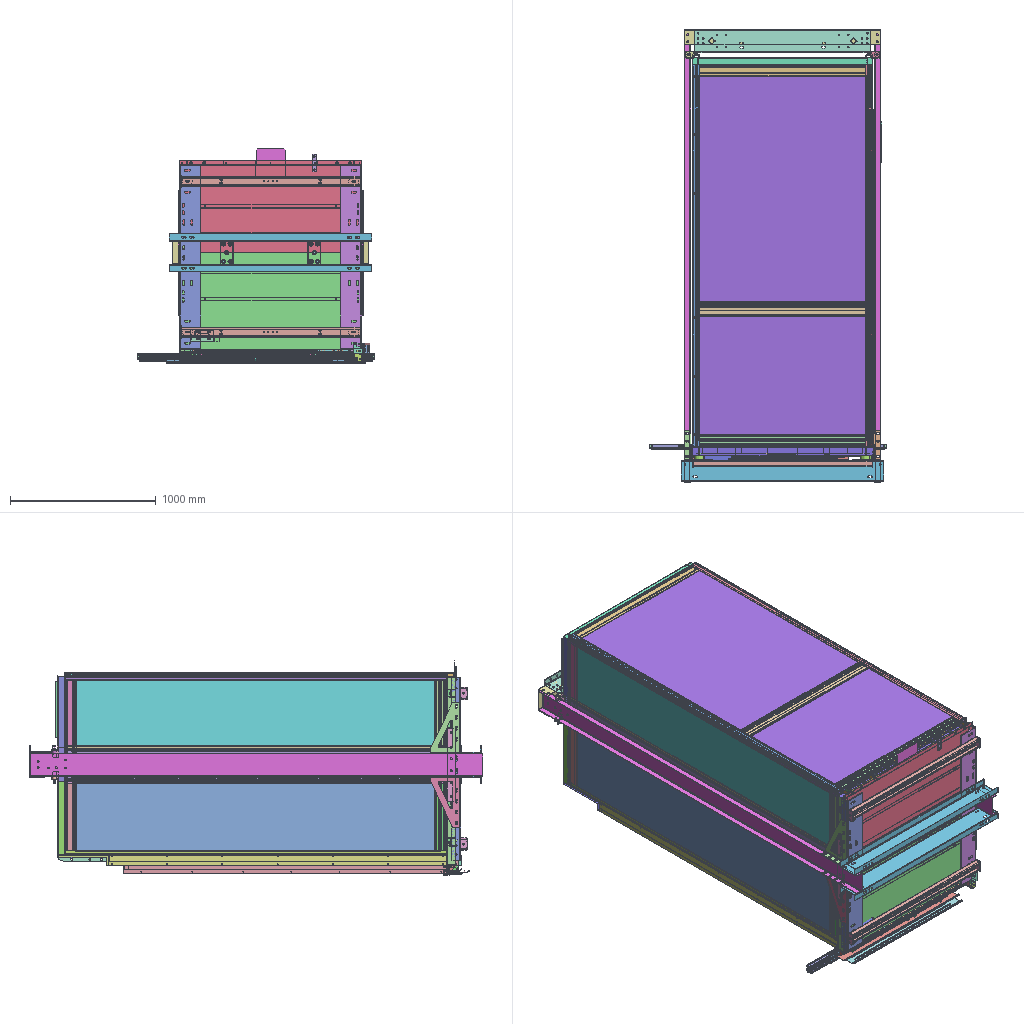Assembly | SolidWorks | 243 different items | 388 placed | box 1620 x 3110 x 1475 mm
Parts list (item | name | quantity | parent item):
1 | 26-3897   减震支架 | x1 | in 3
2 | 26-3897   常规梯专用电缆板A | x1 | in 178
3 | 26-3897   电梯防晃支架 (subassembly) | x1 | in 178
4 | 26-3897   轿厢防晃橡胶垫 | x2 | in 3
5 | 26-3897   轿顶简易盖板 | x1 | in 178
6 | 26-3897   轿顶装饰板前 | x2 | in 178
7 | 26-3897   轿顶装饰板后 | x2 | in 178
8 | 26-3897  CYTJ-B 托架-圆减震垫 | x4 | in 145
9 | 26-3897  地坪尺寸 | x1 | in 175
10 | 26-3897  左前壁下安装板 | x1 | in 15
11 | 26-3897  左前壁主板 | x1 | in 15
12 | 26-3897  左前壁常规加筋 | x1 | in 18
13 | 26-3897  左前壁操纵箱加筋 | x1 | in 18
14 | 26-3897  左前壁操纵箱加筋A | x1 | in 18
15 | 26-3897  左前壁焊件 (subassembly) | x1 | in 18
16 | 26-3897  左前壁盖板 | x1 | in 18
17 | 26-3897  左前壁盖板（齐平盖板） | x1 | in 18
18 | 26-3897  左前壁组件 (subassembly) | x1 | in 175
19 | 26-3897  门楣主板 | x1 | in 23
20 | 26-3897  门楣加筋 | x1 | in 23
21 | 26-3897  门楣加筋（门机门楣安装） | x1 | in 23
22 | 26-3897  门楣安装件 (subassembly) | x1 | in 175
23 | 26-3897  门楣焊件 (subassembly) | x1 | in 22
24 | 26-3897  门楣盖板 | x1 | in 22
25 | 26-3897 COP安装板 | x2 | in 102
26 | 26-3897 DD  吊顶 (subassembly) | x1 | in 176
27 | 26-3897 DD  外协吊顶 | x1 | in 26
28 | 26-3897 DD  星空顶A主板 | x1 | in 32
29 | 26-3897 DD  星空顶A客户确认图 (subassembly) | x1 | in 26
30 | 26-3897 DD  星空顶A封板 | x1 | in 32
31 | 26-3897 DD  星空顶A灯条框 | x1 | in 29
32 | 26-3897 DD  星空顶A焊件 (subassembly) | x1 | in 29
33 | 26-3897 DD  琉璃顶-内板 | x1 | in 36
34 | 26-3897 DD  琉璃顶-客户确认图 (subassembly) | x1 | in 26
35 | 26-3897 DD  琉璃顶-扩散板 | x1 | in 36
36 | 26-3897 DD  琉璃顶-灯罩框架 (subassembly) | x1 | in 34
37 | 26-3897 DD  琉璃顶-焊件总成 (subassembly) | x1 | in 34
38 | 26-3897 DD  琉璃顶-避让钣金 | x1 | in 37
39 | 26-3897 DD  琉璃顶-铝合金边框 | x1 | in 36
40 | 26-3897 DD  琉璃顶主板 | x1 | in 37
41 | 26-3897 DD  白顶-主板 | x1 | in 44
42 | 26-3897 DD  白顶-避让钣金 | x1 | in 44
43 | 26-3897 DD  白顶客户确认图 (subassembly) | x1 | in 26
44 | 26-3897 DD  白顶焊件总成 (subassembly) | x1 | in 43
45 | 26-3897 DD  白顶边框 | x1 | in 43
46 | 26-3897 DD-B1  白顶A主板 | x1 | in 50
47 | 26-3897 DD-B1  白顶A客户确认图 (subassembly) | x1 | in 26
48 | 26-3897 DD-B1  白顶A封板 | x1 | in 50
49 | 26-3897 DD-B1  白顶A灯条框 | x1 | in 47
50 | 26-3897 DD-B1  白顶A焊件 (subassembly) | x1 | in 47
51 | 26-3897 DD-P  白顶-主板 | x1 | in 54
52 | 26-3897 DD-P  白顶-避让钣金右 | x1 | in 54
53 | 26-3897 DD-P  白顶-避让钣金左 | x1 | in 54
54 | 26-3897 DD-P  白顶焊件总成 (subassembly) | x1 | in 43
55 | 26-3897 DD-X1  星空顶A主板 | x1 | in 59
56 | 26-3897 DD-X1  星空顶A客户确认图 (subassembly) | x1 | in 26
57 | 26-3897 DD-X1  星空顶A封板 | x1 | in 59
58 | 26-3897 DD-X1  星空顶A灯条框 | x1 | in 56
59 | 26-3897 DD-X1  星空顶A焊件 (subassembly) | x1 | in 56
60 | 26-3897 OL  70地坎护脚板（旁开） | x2 | in 66
61 | 26-3897 OL  70地坎支架(旁开） | x1 | in 63
62 | 26-3897 OL  70地坎支架 | x1 | in 92
63 | 26-3897 OL  70地坎支架焊件(旁开） (subassembly) | x1 | in 66
64 | 26-3897 OL  70地坎支架筋板(旁开） | x4 | in 63
65 | 26-3897 OL  70地坎支架筋板 | x4 | in 92
66 | 26-3897 OL  70地坎组件（旁开） (subassembly) | x1 | in 96
67 | 26-3897 OL 40-108A地坎 | x1 | in 71
68 | 26-3897 OL 40-108A地坎支架 | x1 | in 70
69 | 26-3897 OL 40-108A地坎支架加筋 | x7 | in 70
70 | 26-3897 OL 40-108A地坎支架焊件 (subassembly) | x1 | in 71
71 | 26-3897 OL 40-108A地坎组件 (subassembly) | x1 | in 96
72 | 26-3897 OL 40-108A护脚板 | x1 | in 71
73 | 26-3897 OL 40地坎支架 | x1 | in 75
74 | 26-3897 OL 40地坎支架加筋 | x6 | in 75
75 | 26-3897 OL 40地坎支架焊件 (subassembly) | x1 | in 76
76 | 26-3897 OL 40地坎组件 (subassembly) | x1 | in 96
77 | 26-3897 OL 40护脚板 | x1 | in 76
78 | 26-3897 OL 40铝合金地坎 | x1 | in 76
79 | 26-3897 OL 60-108D地坎 | x1 | in 80
80 | 26-3897 OL 60-108D地坎组件 (subassembly) | x1 | in 96
81 | 26-3897 OL 60-108D护脚板 | x1 | in 80
82 | 26-3897 OL 60-108D支架 | x1 | in 83
83 | 26-3897 OL 60-108D支架焊件 (subassembly) | x1 | in 80
84 | 26-3897 OL 60-108D支架筋板 | x4 | in 83
85 | 26-3897 OL 60地坎护脚板 | x1 | in 89
86 | 26-3897 OL 60地坎支架 | x1 | in 87
87 | 26-3897 OL 60地坎支架焊件 (subassembly) | x1 | in 89
88 | 26-3897 OL 60地坎支架筋板 | x4 | in 87
89 | 26-3897 OL 60地坎支架组件 (subassembly) | x1 | in 96
90 | 26-3897 OL 60铝合金地坎 | x1 | in 89
91 | 26-3897 OL 70地坎(中分双折) | x1 | in 93
92 | 26-3897 OL 70地坎支架焊件(中分双折) (subassembly) | x1 | in 93
93 | 26-3897 OL 70地坎支架组件(中分双折) (subassembly) | x1 | in 96
94 | 26-3897 OL 70地坎（旁开） | x1 | in 66
95 | 26-3897 OL 70护脚板(中分双折) | x1 | in 93
96 | 26-3897 OL 地坎综合 (subassembly) | x1 | in 176
97 | 26-3897 上梁 | x2 | in 157
98 | 26-3897 下梁 | x2 | in 157
99 | 26-3897 中立柱安装条(右） | x2 | in 101
100 | 26-3897 中立柱安装条(左） | x2 | in 102
101 | 26-3897 中立柱组件(右） (subassembly) | x1 | in 155
102 | 26-3897 中立柱组件(左） (subassembly) | x1 | in 155
103 | 26-3897 中立柱背板(右） | x1 | in 101
104 | 26-3897 中立柱背板(左） | x1 | in 102
105 | 26-3897 中立柱面板(右） | x1 | in 101
106 | 26-3897 中立柱面板(左） | x1 | in 102
107 | 26-3897 侧前玻璃框 | x2 | in 155
108 | 26-3897 侧前玻璃框（Z） | x2 | in 155
109 | 26-3897 侧后玻璃框 | x2 | in 155
110 | 26-3897 侧后玻璃框（Z） | x2 | in 155
111 | 26-3897 侧玻璃框 | x1 | in 155
112 | 26-3897 侧玻璃框（Z） | x1 | in 155
113 | 26-3897 偏心反折DD-X1  星空顶A主板 | x1 | in 116
114 | 26-3897 偏心反折DD-X1  星空顶A封板右 | x1 | in 116
115 | 26-3897 偏心反折DD-X1  星空顶A封板左 | x1 | in 116
116 | 26-3897 偏心反折DD-X1  星空顶A焊件 (subassembly) | x1 | in 56
117 | 26-3897 反折DD-B1  白顶A主板 | x1 | in 119
118 | 26-3897 反折DD-B1  白顶A封板 | x1 | in 119
119 | 26-3897 反折DD-B1  白顶A焊件 (subassembly) | x1 | in 47
120 | 26-3897 反折DD-X1  星空顶A主板 | x1 | in 122
121 | 26-3897 反折DD-X1  星空顶A封板 | x1 | in 122
122 | 26-3897 反折DD-X1  星空顶A焊件 (subassembly) | x1 | in 56
123 | 26-3897 台阶螺钉 | x28 | in 101, 102
124 | 26-3897 右前壁一体操纵箱 | x1 | in 175
125 | 26-3897 右前壁下安装板 | x1 | in 130
126 | 26-3897 右前壁主板 | x1 | in 130
127 | 26-3897 右前壁常规加筋 | x1 | in 133
128 | 26-3897 右前壁操纵箱加筋 | x1 | in 133
129 | 26-3897 右前壁操纵箱加筋A | x1 | in 133
130 | 26-3897 右前壁焊件 (subassembly) | x1 | in 133
131 | 26-3897 右前壁盖板 | x1 | in 133
132 | 26-3897 右前壁盖板（齐平盖板） | x1 | in 133
133 | 26-3897 右前壁组件 (subassembly) | x1 | in 175
134 | 26-3897 后壁玻璃框扶手 | x1 | in 155
135 | 26-3897 后壁玻璃框扶手（Z） | x1 | in 155
136 | 26-3897 后玻璃框 | x1 | in 155
137 | 26-3897 后玻璃框（Z） | x1 | in 155
138 | 26-3897 外购A-1 电梯防晃卡板 | x4 | in 178
139 | 26-3897 左前壁一体操纵箱 | x1 | in 175
140 | 26-3897 托架中梁B | x1 | -
141 | 26-3897 托架中梁B加筋 | x1 | -
142 | 26-3897 托架侧梁 | x2 | in 145
143 | 26-3897 托架电缆支架A | x1 | -
144 | 26-3897 托架电缆支架B | x1 | -
145 | 26-3897 托架组件 (subassembly) | x1 | in 187
146 | 26-3897 托架边梁 | x1 | in 147
147 | 26-3897 托架边梁焊件 (subassembly) | x1 | in 145
148 | 26-3897 旁开门前壁主板 | x1 | in 152
149 | 26-3897 旁开门前壁加筋 | x2 | in 152
150 | 26-3897 旁开门前壁垫板 | x2 | in 153
151 | 26-3897 旁开门前壁安装板 | x1 | in 152
152 | 26-3897 旁开门前壁焊件 (subassembly) | x1 | in 153
153 | 26-3897 旁开门前壁组件 (subassembly) | x1 | in 175
154 | 26-3897 标注图勿动 (subassembly) | x1 | in 155
155 | 26-3897 框架A (subassembly) | x1 | in 156
156 | 26-3897 框架S (subassembly) | x1 | in 175
157 | 26-3897 梁组件 (subassembly) | x1 | in 187
158 | 26-3897 横向加筋 | x2 | in 180
159 | 26-3897 深渊镜-单面镜 | x1 | in 163
160 | 26-3897 深渊镜-外型材 | x1 | in 163
161 | 26-3897 深渊镜-镜子 | x1 | in 163
162 | 26-3897 深渊镜客户确认图 (subassembly) | x1 | in 26
163 | 26-3897 深渊镜核心组件 (subassembly) | x1 | in 162
164 | 26-3897 深渊镜横向型材 | x2 | in 163
165 | 26-3897 深渊镜纵向型材 | x2 | in 163
166 | 26-3897 深渊顶-主板 | x1 | in 168
167 | 26-3897 深渊顶-避让钣金 | x1 | in 168
168 | 26-3897 深渊顶焊件总成 (subassembly) | x1 | in 162
169 | 26-3897 磁栅尺支架 | x2 | in 180
170 | 26-3897 立柱灯带槽(右） | x2 | in 101
171 | 26-3897 立柱灯带槽(左） | x2 | in 102
172 | 26-3897 立梁 | x2 | in 157
173 | 26-3897 纵向加筋 | x2 | in 180
174 | 26-3897 踏板 | x1 | in 176
175 | 26-3897 轿厢总成A (subassembly) | x1 | in 176
176 | 26-3897 轿厢总成B (subassembly) | x1 | -
177 | 26-3897 轿顶主板 | x1 | in 180
178 | 26-3897 轿顶安装总成 (subassembly) | x1 | in 175
179 | 26-3897 轿顶横向边梁 | x1 | in 180
180 | 26-3897 轿顶焊接总成 (subassembly) | x1 | in 178
181 | 26-3897 轿顶纵向边梁 | x1 | in 180
182 | 26-3897 轿顶防晃支架 | x2 | in 180
183 | 26-3897 铝合金地坎 | x1 | in 176
184 | 26-3897 门机支架 | x2 | in 180
185 | 26-3897 门机支架A | x1 | in 180
186 | 26-3897 飞机板 | x1 | in 157
187 | 26-3897 龙门架组件 (subassembly) | x1 | -
188 | 26-3897-扶手 | x1 | in 176
189 | 26-3897A   称重板 | x1 | in 197
190 | 26-3897A   轿底电缆固定板 | x1 | in 197
191 | 26-3897A  侧筋板 | x22 | in 197
192 | 26-3897A  后筋板 | x6 | in 197
193 | 26-3897A  轿底两侧加强筋 | x1 | in 197
194 | 26-3897A  轿底主板 | x1 | in 197
195 | 26-3897A  轿底加筋 | x6 | in 197
196 | 26-3897A  轿底横向加强筋 | x1 | in 197
197 | 26-3897A  轿底焊接总成 (subassembly) | x1 | in 198
198 | 26-3897A  轿底装配总成 (subassembly) | x1 | in 175
199 | 26-3897B  轿底电缆固定板 | x1 | in 211
200 | 26-3897B 侧筋板A | x8 | in 211
201 | 26-3897B 侧筋板B | x8 | in 211
202 | 26-3897B 后筋板 | x6 | in 211
203 | 26-3897B 轿底两侧加强筋 | x1 | in 211
204 | 26-3897B 轿底中间加筋A | x2 | in 211
205 | 26-3897B 轿底中间加筋B | x4 | in 211
206 | 26-3897B 轿底主板 | x1 | in 211
207 | 26-3897B 轿底安装孔内加厚板 | x2 | in 211
208 | 26-3897B 轿底安装孔外加厚板 | x2 | in 211
209 | 26-3897B 轿底安装总成 (subassembly) | x1 | in 175
210 | 26-3897B 轿底横向加强筋 | x1 | in 211
211 | 26-3897B 轿底焊接总成 (subassembly) | x1 | in 209
212 | 26-3897B 轿底盖板 | x1 | in 209
213 | 26-3897B 轿底缓冲器加筋 | x2 | in 211
214 | 26-3897上梁A | x1 | in 157
215 | hex nuts, style 1-grades ab gb | x1 | -
216 | hexagon weld nuts gb | x1 | -
217 | plain washers--product grade c gb | x1 | -
218 | 封板 | x4 | in 145
219 | 美奥10.1英寸控制柜148x265 | x1 | in 156
220 | 镜向26-3897   减震支架 | x1 | in 222
221 | 镜向26-3897   减震支架1 | x1 | in 223
222 | 镜向26-3897   电梯防晃支架 (subassembly) | x1 | in 178
223 | 镜向26-3897   电梯防晃支架1 (subassembly) | x1 | in 178
224 | 镜向26-3897   轿厢防晃橡胶垫 | x2 | in 222
225 | 镜向26-3897   轿厢防晃橡胶垫1 | x2 | in 223
226 | 镜向26-3897  左前壁下安装板 | x1 | in 15
227 | 镜向26-3897  门楣加筋 | x1 | in 23
228 | 镜向26-3897  门楣加筋（门机门楣安装） | x1 | in 23
229 | 镜向26-3897 侧玻璃框 | x1 | in 155
230 | 镜向26-3897 侧玻璃框（Z） | x1 | in 155
231 | 镜向26-3897 右前壁下安装板 | x1 | in 130
232 | 镜向26-3897 托架边梁 | x1 | in 233
233 | 镜向26-3897 托架边梁焊件 (subassembly) | x1 | in 145
234 | 镜向26-3897 旁开门前壁安装板 | x1 | in 152
235 | 镜向26-3897 轿顶纵向边梁 | x1 | in 180
236 | 镜向26-3897 飞机板 | x1 | in 157
237 | 镜向26-3897 飞机板1 | x1 | in 157
238 | 镜向26-3897A  轿底两侧加强筋 | x1 | in 197
239 | 镜向26-3897B 轿底两侧加强筋 | x1 | in 211
240 | 镜向镜向26-3897   减震支架 | x1 | in 241
241 | 镜向镜向26-3897   电梯防晃支架 (subassembly) | x1 | in 178
242 | 镜向镜向26-3897   轿厢防晃橡胶垫 | x2 | in 241
243 | 镜向镜向26-3897 飞机板 | x1 | in 157
Mates (type | each side: item.copy, entity, surface, feature), first 723 of 755 lines:
In the top assembly
Coincident | 176.1 plane | 187.1 plane | 2 times
Coincident | 238.1 face plane 26-3897A  轿底两侧加强筋_镜向 | 8.1 face plane 凸台-拉伸1
In subassembly 187
Coincident | 187.2 face | 187.2 face
Concentric | 187.2 face | 187.2 face
Coincident | 157.1 plane | 187.2 plane | 3 times
Coincident | 145.1 plane | 187.2 plane | 2 times
DistanceDim | 172.1 face plane 基体-法兰1 | 146.1 face plane 基体-法兰1
In subassembly 157
Coincident | 157.2 face | 157.2 face
Concentric | 157.2 face | 157.2 face
Coincident | 97.1 plane | 157.2 plane
Coincident | 97.1 face | 157.2 plane
Coincident | 172.2 plane | 157.2 plane
Coincident | 97.1 face | 172.2 face plane 基体-法兰1 | 2 times
DistanceDim | 97.1 face | 172.2 face plane 基体-法兰1
Coincident | 172.2 face plane 基体-法兰1 | 186.1 face plane 基体-法兰1 | 2 times
Coincident | 214.1 plane | 157.2 plane | 3 times
DistanceDim | 214.1 face plane 基体-法兰1 | 172.2 face plane 基体-法兰1
DistanceDim | 172.2 face plane 基体-法兰1 | 214.1 face plane 基体-法兰1
DistanceDim | 186.1 face plane 基体-法兰1 | 172.2 face plane 基体-法兰1
Coincident | 172.2 face plane 基体-法兰1 | 98.1 face plane 基体-法兰1
Coincident | 98.1 plane | 157.2 plane
DistanceDim | 236.1 face plane 26-3897 飞机板_镜向 | 98.1 face plane 基体-法兰1
In subassembly 145
Coincident | 145.2 face | 145.2 face
Concentric | 145.2 face | 145.2 face
Coincident | 147.1 plane | 145.2 plane
Coincident | 146.2 face plane 基体-法兰1 | 145.2 plane
Coincident | 142.1 plane | 145.2 plane
Coincident | 146.2 face plane 基体-法兰1 | 142.1 face plane 基体-法兰1
Coincident | assembly plane | 145.2 plane | 4 times
Coincident | assembly face | 146.2 face plane 基体-法兰1
DistanceDim | 146.2 face plane 基体-法兰1 | 232.1 face plane 26-3897 托架边梁_镜向
Parallel | 146.2 face plane 基体-法兰1 | assembly face
Coincident | 146.2 face plane 基体-法兰1 | assembly face | 2 times
Parallel | assembly face | assembly face
Coincident | 146.2 face plane 基体-法兰1 | 145.2 face
Coincident | 146.2 face plane 基体-法兰1 | 8.2 face plane 凸台-拉伸1
DistanceDim | 142.1 face plane 基体-法兰1 | 146.2 face plane 基体-法兰1
DistanceDim | 146.2 face plane 基体-法兰1 | 8.2 face cylinder 凸台-拉伸3
DistanceDim | 8.2 face cylinder 凸台-拉伸3 | 146.2 face plane 基体-法兰1
Coincident | 142.1 face plane 基体-法兰1 | 218.1 face plane 凸台-拉伸1
Coincident | 142.1 edge | 218.1 face plane 凸台-拉伸1
DistanceDim | 218.1 face plane 凸台-拉伸1 | 142.1 face plane 基体-法兰1
In subassembly 147
Coincident | 147.2 face | 147.2 face
Concentric | 147.2 face | 147.2 face
Coincident | 146.3 plane | 147.2 plane | 3 times
In subassembly 176
Coincident | 176.2 face | 176.2 face
Concentric | 176.2 face | 176.2 face
Coincident | 175.1 plane | 176.2 plane | 3 times
Coincident | 194.1 face plane 基体-法兰1 | 174.1 face plane 凸台-拉伸1 | 2 times
Coincident | 154.1 plane | 174.1 plane
Coincident | 194.1 face plane 基体-法兰1 | 73.1 face plane 基体-法兰1
DistanceDim | 78.1 face plane 凸台-拉伸1 | 194.1 face plane 基体-法兰1
Coincident | 154.1 plane | 96.1 plane
Coincident | 194.1 face plane 基体-法兰1 | 183.1 face plane 凸台-拉伸1
Coincident | 78.1 face plane 凸台-拉伸1 | 183.1 face plane 凸台-拉伸1
Coincident | 183.1 plane | 176.2 plane
Coincident | 177.1 face plane 基体-法兰1 | 27.1 face plane 凸台-拉伸1
DistanceDim | 109.1 face plane 20款轿厢 20款轿厢-下横档(1) | 27.1 face plane 凸台-拉伸1
DistanceDim | 136.1 face plane 20款轿厢 20款轿厢-后边框(1) | 27.1 face plane 凸台-拉伸1
Coincident | 135.1 face plane 玻璃 | 188.1 face plane 凸台-拉伸2
In subassembly 96
Coincident | 96.2 face | 96.2 face
Concentric | 96.2 face | 96.2 face
Coincident | 76.1 plane | 96.2 plane | 3 times
Coincident | 73.2 face plane 基体-法兰1 | 62.1 face plane 基体-法兰1
Coincident | 78.2 face plane 凸台-拉伸1 | 91.1 face plane 凸台-拉伸1
Coincident | 93.1 plane | 96.2 plane
Coincident | 89.1 plane | 96.2 plane
Coincident | 73.2 face plane 基体-法兰1 | 86.1 face plane 基体-法兰1
Coincident | 78.2 face plane 凸台-拉伸1 | 90.1 face plane 凸台-拉伸1
Coincident | 73.2 face plane 基体-法兰1 | 61.1 face plane 基体-法兰1
Coincident | 78.2 face plane 凸台-拉伸1 | 94.1 face plane 凸台-拉伸1
Coincident | 73.2 face plane 基体-法兰1 | 79.1 face plane 凸台-拉伸1
Coincident | 80.1 plane | 96.2 plane
Coincident | 78.2 face plane 凸台-拉伸1 | 67.1 face plane 凸台-拉伸1
Coincident | 73.2 face plane 基体-法兰1 | 68.1 face plane 基体-法兰1
Coincident | 71.1 plane | 96.2 plane
Coincident | 78.2 face plane 凸台-拉伸1 | 79.1 face plane 凸台-拉伸1
In subassembly 76
Coincident | 76.2 face | 76.2 face
Concentric | 76.2 face | 76.2 face
Coincident | 75.1 plane | 76.2 plane | 3 times
Coincident | 73.3 face plane 基体-法兰1 | 78.3 face plane 凸台-拉伸1 | 2 times
Coincident | 78.3 plane | 76.2 plane
Coincident | 73.3 face plane 基体-法兰1 | 77.1 face plane 基体-法兰1
Coincident | 77.1 plane | 76.2 plane
Coincident | 78.3 face plane 凸台-拉伸1 | 77.1 face plane 基体-法兰1
In subassembly 75
Coincident | 75.2 face | 75.2 face
Concentric | 75.2 face | 75.2 face
Coincident | 73.4 plane | 75.2 plane | 2 times
Coincident | 73.4 face plane 基体-法兰1 | 75.2 plane
Coincident | 73.4 face plane 基体-法兰1 | 74.1 face plane 凸台-拉伸1 | 2 times
DistanceDim | 73.4 face plane 基体-法兰1 | 74.1 edge
In subassembly 93
Coincident | 93.2 face | 93.2 face
Concentric | 93.2 face | 93.2 face
Coincident | 91.2 plane | 93.2 plane | 3 times
Coincident | 95.1 plane | 93.2 plane
Coincident | 91.2 face plane 凸台-拉伸1 | 93.2 plane
Coincident | 91.2 face plane 凸台-拉伸1 | 62.2 face plane 基体-法兰1 | 2 times
Coincident | 92.1 plane | 93.2 plane
Coincident | 95.1 face plane 基体-法兰1 | 62.2 face plane 基体-法兰1
DistanceDim | 95.1 face plane 基体-法兰1 | 62.2 face plane 基体-法兰1
In subassembly 92
Coincident | 92.2 face | 92.2 face
Concentric | 92.2 face | 92.2 face
Coincident | 62.3 plane | 92.2 plane
Coincident | 62.3 face plane 基体-法兰1 | 92.2 plane | 2 times
Coincident | 62.3 face plane 基体-法兰1 | 65.1 face plane 凸台-拉伸1 | 2 times
DistanceDim | 65.1 face plane 凸台-拉伸1 | 62.3 face plane 基体-法兰1
Coincident | 62.3 face plane 基体-法兰1 | 65.2 face plane 凸台-拉伸1 | 2 times
DistanceDim | 62.3 face cylinder 切除-拉伸2 | 65.2 face plane 凸台-拉伸1
In subassembly 80
Coincident | 80.2 face | 80.2 face
Concentric | 80.2 face | 80.2 face
Coincident | 79.2 plane | 80.2 plane | 3 times
Coincident | 79.2 face plane 凸台-拉伸2 | 82.1 face plane 基体-法兰1
Coincident | 83.1 plane | 80.2 plane
Coincident | 79.2 face plane 凸台-拉伸1 | 82.1 face plane 基体-法兰1
Coincident | 82.1 face plane 基体-法兰1 | 81.1 face plane 基体-法兰1
Coincident | 81.1 plane | 80.2 plane
DistanceDim | 79.2 face plane 凸台-拉伸2 | 81.1 face plane 基体-法兰1
In subassembly 83
Coincident | 83.2 face | 83.2 face
Concentric | 83.2 face | 83.2 face
Coincident | 82.2 plane | 83.2 plane
Coincident | 82.2 face plane 基体-法兰1 | 83.2 plane | 2 times
Coincident | 82.2 face plane 基体-法兰1 | 84.1 face plane 凸台-拉伸1 | 2 times
DistanceDim | 84.1 face plane 凸台-拉伸1 | 82.2 face plane 基体-法兰1
In subassembly 66
Coincident | 66.1 face | 66.1 face
Concentric | 66.1 face | 66.1 face
Coincident | 94.2 plane | 66.1 plane | 3 times
Coincident | 94.2 face plane 凸台-拉伸1 | 61.2 face plane 基体-法兰1 | 2 times
Coincident | 61.2 face plane 基体-法兰1 | 60.1 face plane 基体-法兰1
Coincident | 63.1 plane | 60.1 plane
DistanceDim | 61.2 face plane 基体-法兰1 | 60.1 face plane 基体-法兰1
Coincident | 94.2 face plane 凸台-拉伸1 | 60.2 face plane 基体-法兰1 | 2 times
Coincident | 60.1 face plane 基体-法兰1 | 60.2 face plane 基体-法兰1
In subassembly 63
Coincident | 63.2 face | 63.2 face
Concentric | 63.2 face | 63.2 face
Coincident | 61.3 plane | 63.2 plane
Coincident | 61.3 face plane 基体-法兰1 | 63.2 plane | 2 times
Coincident | 61.3 face plane 基体-法兰1 | 64.1 face plane 凸台-拉伸1 | 2 times
DistanceDim | 64.1 face plane 凸台-拉伸1 | 61.3 face plane 基体-法兰1
Coincident | 61.3 face plane 基体-法兰1 | 64.2 face plane 凸台-拉伸1 | 2 times
DistanceDim | 61.3 face cylinder 切除-拉伸2 | 64.2 face plane 凸台-拉伸1
In subassembly 89
Coincident | 89.2 face | 89.2 face
Concentric | 89.2 face | 89.2 face
Coincident | 87.1 plane | 89.2 plane | 3 times
Coincident | 85.1 face plane 基体-法兰1 | 86.2 face plane 基体-法兰1
Coincident | 85.1 plane | 89.2 plane
Slot | 85.1 face cylinder 切除-拉伸1 | 86.2 face cylinder 切除-拉伸3
Coincident | 86.2 face plane 基体-法兰1 | 90.2 face plane 凸台-拉伸1 | 2 times
Coincident | 90.2 plane | 89.2 plane
In subassembly 87
Coincident | 87.2 face | 87.2 face
Concentric | 87.2 face | 87.2 face
Coincident | 86.3 plane | 87.2 plane
Coincident | 86.3 face plane 基体-法兰1 | 87.2 plane | 2 times
Coincident | 86.3 face plane 基体-法兰1 | 88.1 face plane 凸台-拉伸1 | 2 times
DistanceDim | 88.1 face plane 凸台-拉伸1 | 86.3 face plane 基体-法兰1
In subassembly 71
Coincident | 71.2 face | 71.2 face
Concentric | 71.2 face | 71.2 face
Coincident | 67.2 plane | 71.2 plane | 3 times
Coincident | 70.1 plane | 71.2 plane
Coincident | 67.2 face plane 凸台-拉伸1 | 68.2 face plane 基体-法兰1
Coincident | 67.2 face plane 凸台-拉伸2 | 68.2 face plane 基体-法兰1
Coincident | 68.2 face plane 基体-法兰1 | 72.1 face plane 基体-法兰1
Coincident | 72.1 plane | 71.2 plane
DistanceDim | 67.2 face plane 凸台-拉伸1 | 72.1 face plane 基体-法兰1
In subassembly 70
Coincident | 70.2 face | 70.2 face
Concentric | 70.2 face | 70.2 face
Coincident | 68.3 plane | 70.2 plane | 2 times
Coincident | 68.3 face plane 基体-法兰1 | 70.2 plane
Coincident | 68.3 face plane 基体-法兰1 | 69.1 face plane 凸台-拉伸1 | 3 times
Coincident | 68.3 face plane 基体-法兰1 | 69.2 face plane 凸台-拉伸1 | 2 times
DistanceDim | 70.2 plane | 69.2 face plane 凸台-拉伸1
Coincident | 68.3 face plane 基体-法兰1 | 69.3 face plane 凸台-拉伸1 | 2 times
DistanceDim | 68.3 face plane 切除-拉伸2 | 69.3 face plane 凸台-拉伸1
In subassembly 26
Coincident | 26.1 face | 26.1 face
Concentric | 26.1 face | 26.1 face
Coincident | 27.2 plane | 26.1 plane | 2 times
Coincident | 27.2 face plane 凸台-拉伸1 | 26.1 plane
Coincident | 27.2 face plane 凸台-拉伸1 | 41.1 face plane 基体-法兰1
Coincident | 43.1 plane | 26.1 plane | 2 times
Coincident | 29.1 plane | 26.1 plane | 2 times
Coincident | 27.2 face plane 凸台-拉伸1 | 28.1 face plane 基体-法兰1
Coincident | 27.2 face plane 凸台-拉伸1 | 40.1 face plane 基体-法兰1
Coincident | 34.1 plane | 26.1 plane | 2 times
Coincident | 47.1 plane | 26.1 plane | 2 times
Coincident | 27.2 face plane 凸台-拉伸1 | 46.1 face plane 基体-法兰1
Coincident | 56.1 plane | 26.1 plane | 2 times
Coincident | 27.2 face plane 凸台-拉伸1 | 55.1 face plane 基体-法兰1
Coincident | 162.1 plane | 26.1 plane | 2 times
Coincident | 41.1 face plane 基体-法兰1 | 166.1 face plane 基体-法兰1
In subassembly 34
Coincident | 34.2 face | 34.2 face
Concentric | 34.2 face | 34.2 face
Coincident | 37.1 plane | 34.2 plane | 2 times
Coincident | 36.1 plane | 34.2 plane | 2 times
Coincident | 33.1 face plane 凸台-拉伸1 | 40.2 face plane 边线-法兰2
Coincident | 40.2 face plane 基体-法兰1 | 34.2 plane
In subassembly 37
Coincident | 37.2 face | 37.2 face
Concentric | 37.2 face | 37.2 face
Coincident | 40.3 face plane 基体-法兰1 | 37.2 plane
Coincident | 40.3 plane | 37.2 plane | 2 times
Coincident | 40.3 face plane 基体-法兰1 | 38.1 edge
Coincident | 40.3 face plane 正风机 | 38.1 edge | 2 times
Width | 40.3 face plane 正风机 | 40.3 face plane 正风机 | 38.1 face plane 边线-法兰1 | 38.1 face plane 镜向1
Coincident | 40.3 face plane 基体-法兰1 | 38.2 edge
Coincident | 40.3 face | 38.2 edge | 2 times
Width | 38.2 face | 38.2 face | 40.3 face | 40.3 face
In subassembly 36
Coincident | 39.1 plane | 36.2 plane | 2 times
Coincident | 39.1 face plane 发光背板型材 边框(1) | 36.2 plane
Coincident | 35.1 plane | 36.2 plane | 2 times
Coincident | 35.1 face plane 凸台-拉伸1 | 39.1 edge
Coincident | 39.1 face plane 发光背板型材 边框(1) | 33.2 face plane 凸台-拉伸1
Coincident | 33.2 plane | 36.2 plane | 2 times
In subassembly 56
Coincident | 56.2 face | 56.2 face
Concentric | 56.2 face | 56.2 face
Coincident | 59.1 plane | 56.2 plane | 2 times
Coincident | 55.2 face plane 基体-法兰1 | 56.2 plane
Coincident | 58.1 plane | 56.2 plane | 2 times
Coincident | 58.1 face plane 吊顶型材 星空顶型材（250403）(1) | 55.2 face plane 边线-法兰2
Coincident | 122.1 plane | 56.2 plane | 2 times
Coincident | 58.1 face plane 吊顶型材 星空顶型材（250403）(1) | 120.1 face plane 边线-法兰2
Coincident | 58.1 face plane 吊顶型材 星空顶型材（250403）(1) | 113.1 face plane 边线-法兰2
Coincident | 116.1 plane | 56.2 plane | 2 times
In subassembly 122
Coincident | 122.2 face | 122.2 face
Concentric | 122.2 face | 122.2 face
Coincident | 120.2 plane | 122.2 plane | 2 times
Coincident | 120.2 face plane 基体-法兰1 | 122.2 plane
Width | 121.1 face plane 镜向1 | 121.1 face plane 边线-法兰1 | 120.2 face plane 正风机 | 120.2 face plane 正风机
Coincident | 120.2 face plane 基体-法兰1 | 121.1 edge
Coincident | 120.2 face plane 正风机 | 121.1 edge | 2 times
Width | 121.2 face | 121.2 face | 120.2 face | 120.2 face
Coincident | 120.2 face plane 基体-法兰1 | 121.2 edge
Coincident | 120.2 face | 121.2 edge | 2 times
In subassembly 59
Coincident | 59.2 face | 59.2 face
Concentric | 59.2 face | 59.2 face
Coincident | 55.3 plane | 59.2 plane | 2 times
Coincident | 55.3 face plane 基体-法兰1 | 59.2 plane
Width | 57.1 face plane 镜向1 | 57.1 face plane 边线-法兰1 | 55.3 face plane 正风机 | 55.3 face plane 正风机
Coincident | 55.3 face plane 基体-法兰1 | 57.1 edge
Coincident | 55.3 face plane 正风机 | 57.1 edge | 2 times
Width | 57.2 face | 57.2 face | 55.3 face | 55.3 face
Coincident | 55.3 face plane 基体-法兰1 | 57.2 edge
Coincident | 55.3 face | 57.2 edge | 2 times
In subassembly 116
Coincident | 116.2 face | 116.2 face
Concentric | 116.2 face | 116.2 face
Coincident | 113.2 plane | 116.2 plane | 2 times
Coincident | 113.2 face plane 基体-法兰1 | 116.2 plane
Coincident | 113.2 face plane 切口 | 115.1 edge | 2 times
Coincident | 113.2 face plane 边线-法兰1 | 115.1 face plane 基体-法兰1
Coincident | 113.2 face plane 基体-法兰1 | 115.1 edge
Coincident | 113.2 face plane 边线-法兰1 | 114.1 edge
Coincident | 113.2 face plane 边线-法兰1 | 114.1 face plane 基体-法兰1
Coincident | 113.2 face plane 基体-法兰1 | 114.1 edge
Coincident | 113.2 face plane 切口 | 114.1 edge
In subassembly 43
Coincident | 43.2 face | 43.2 face
Concentric | 43.2 face | 43.2 face
Coincident | 44.1 plane | 43.2 plane | 2 times
Coincident | 41.2 face plane 基体-法兰1 | 43.2 plane
Coincident | 45.1 plane | 43.2 plane | 2 times
Coincident | 41.2 face plane 边线-法兰2 | 45.1 face plane 发光背板型材 边框(1)
Coincident | 54.1 plane | 43.2 plane | 2 times
Coincident | 45.1 face plane 发光背板型材 边框(1) | 51.1 face plane 边线-法兰2
In subassembly 44
Coincident | 44.2 face | 44.2 face
Concentric | 44.2 face | 44.2 face
Coincident | 41.3 plane | 44.2 plane | 2 times
Coincident | 41.3 face plane 基体-法兰1 | 44.2 plane
Coincident | 42.1 plane | 44.2 plane
Coincident | 41.3 face plane 基体-法兰1 | 42.1 edge
Coincident | 41.3 face plane 正风机 | 42.1 edge | 2 times
Width | 42.2 face | 42.2 face | 41.3 face | 41.3 face
Coincident | 41.3 face | 42.2 edge | 2 times
Coincident | 41.3 face plane 基体-法兰1 | 42.2 edge
In subassembly 54
Coincident | 54.2 face | 54.2 face
Concentric | 54.2 face | 54.2 face
Coincident | 51.2 plane | 54.2 plane | 2 times
Coincident | 51.2 face plane 基体-法兰1 | 54.2 plane
Coincident | 51.2 face plane 基体-法兰1 | 53.1 edge
Coincident | 51.2 face plane 边线-法兰1 | 53.1 face plane 基体-法兰1
Coincident | 51.2 face plane 边线-法兰1 | 53.1 edge
Coincident | 51.2 face plane 正风机 | 53.1 edge
Coincident | 51.2 face plane 边线-法兰1 | 52.1 face plane 基体-法兰1
Coincident | 51.2 face plane 基体-法兰1 | 52.1 edge
Coincident | 51.2 face plane 边线-法兰1 | 52.1 edge
Coincident | 51.2 face plane 正风机 | 52.1 edge
In subassembly 162
Coincident | 162.2 face | 162.2 face
Concentric | 162.2 face | 162.2 face
Coincident | 163.1 plane | 162.2 plane | 2 times
Coincident | 168.1 plane | 162.2 plane | 2 times
Coincident | 166.2 face plane 边线-法兰2 | 160.1 face plane 扫描4
In subassembly 168
Coincident | 168.2 face | 168.2 face
Concentric | 168.2 face | 168.2 face
Coincident | 166.3 plane | 168.2 plane | 2 times
Coincident | 166.3 face plane 基体-法兰1 | 168.2 plane
Coincident | 167.1 plane | 168.2 plane
Coincident | 166.3 face plane 基体-法兰1 | 167.1 edge
Coincident | 166.3 face plane 切除-拉伸4 | 167.1 edge | 2 times
In subassembly 163
Coincident | 165.1 face plane 凸台-拉伸1 | 164.1 face plane 凸台-拉伸1 | 3 times
Coincident | 164.1 face plane 凸台-拉伸1 | 165.2 face plane 凸台-拉伸1 | 3 times
Coincident | 165.2 face plane 凸台-拉伸1 | 164.2 face plane 凸台-拉伸1 | 3 times
Coincident | 165.1 face plane 凸台-拉伸1 | 159.1 face plane 凸台-拉伸1
Coincident | 165.2 face plane 凸台-拉伸1 | 159.1 face plane 凸台-拉伸1 | 2 times
Coincident | 164.1 face plane 凸台-拉伸1 | 161.1 face plane 凸台-拉伸1
Coincident | 165.1 face plane 凸台-拉伸1 | 161.1 face plane 凸台-拉伸1
Coincident | 164.2 face plane 凸台-拉伸1 | 161.1 face plane 凸台-拉伸1
Coincident | 160.2 plane | 163.2 plane | 2 times
Coincident | 159.1 plane | 163.2 plane | 2 times
Coincident | 161.1 face plane 凸台-拉伸1 | 160.2 face plane 扫描4
Coincident | 159.1 face plane 凸台-拉伸1 | 163.2 plane
In subassembly 47
Coincident | 47.2 face | 47.2 face
Concentric | 47.2 face | 47.2 face
Coincident | 50.1 plane | 47.2 plane | 2 times
Coincident | 46.2 face plane 基体-法兰1 | 47.2 plane
Coincident | 49.1 plane | 47.2 plane | 2 times
Coincident | 49.1 face plane 吊顶型材 星空顶型材（250403）(1) | 46.2 face plane 边线-法兰2
Coincident | 119.1 plane | 47.2 plane | 2 times
Coincident | 49.1 face plane 吊顶型材 星空顶型材（250403）(1) | 117.1 face plane 边线-法兰2
In subassembly 119
Coincident | 119.2 face | 119.2 face
Concentric | 119.2 face | 119.2 face
Coincident | 117.2 plane | 119.2 plane | 2 times
Coincident | 117.2 face plane 基体-法兰1 | 119.2 plane
Width | 118.1 face plane 镜向1 | 118.1 face plane 边线-法兰1 | 117.2 face plane 正风机 | 117.2 face plane 正风机
Coincident | 117.2 face plane 基体-法兰1 | 118.1 edge
Coincident | 117.2 face plane 正风机 | 118.1 edge | 2 times
Width | 118.2 face | 118.2 face | 117.2 face | 117.2 face
Coincident | 117.2 face plane 基体-法兰1 | 118.2 edge
Coincident | 117.2 face | 118.2 edge | 2 times
In subassembly 50
Coincident | 50.2 face | 50.2 face
Concentric | 50.2 face | 50.2 face
Coincident | 46.3 plane | 50.2 plane | 2 times
Coincident | 46.3 face plane 基体-法兰1 | 50.2 plane
Width | 48.1 face plane 镜向1 | 48.1 face plane 边线-法兰1 | 46.3 face plane 正风机 | 46.3 face plane 正风机
Coincident | 46.3 face plane 基体-法兰1 | 48.1 edge
Coincident | 46.3 face plane 正风机 | 48.1 edge | 2 times
Width | 48.2 face | 48.2 face | 46.3 face | 46.3 face
Coincident | 46.3 face plane 基体-法兰1 | 48.2 edge
Coincident | 46.3 face | 48.2 edge | 2 times
In subassembly 29
Coincident | 29.2 face | 29.2 face
Concentric | 29.2 face | 29.2 face
Coincident | 31.1 plane | 29.2 plane | 2 times
Coincident | 31.1 face plane 自定义 灯条型材(1) | 29.2 plane
Coincident | 28.2 face plane 边线-法兰2 | 31.1 face plane 自定义 灯条型材(1)
Coincident | 32.1 plane | 29.2 plane | 2 times
In subassembly 32
Coincident | 32.2 face | 32.2 face
Concentric | 32.2 face | 32.2 face
Coincident | 28.3 plane | 32.2 plane | 2 times
Coincident | 28.3 face plane 基体-法兰1 | 32.2 plane
Width | 30.1 face plane 镜向1 | 30.1 face plane 边线-法兰1 | 28.3 face plane 正风机 | 28.3 face plane 正风机
Coincident | 28.3 face plane 基体-法兰1 | 30.1 edge
Coincident | 28.3 face plane 正风机 | 30.1 edge | 2 times
Width | 30.2 face | 30.2 face | 28.3 face | 28.3 face
Coincident | 28.3 face plane 基体-法兰1 | 30.2 edge
Coincident | 28.3 face | 30.2 edge | 2 times
In subassembly 175
Coincident | 175.2 face | 175.2 face
Concentric | 175.2 face | 175.2 face
Coincident | 156.1 plane | 175.2 plane | 3 times
Coincident | 178.1 plane | 175.2 plane | 2 times
Coincident | 136.2 face plane 20款轿厢 20款轿厢-上横档(1) | 177.2 face plane 基体-法兰1
Coincident | 198.1 plane | 175.2 plane | 2 times
Coincident | 136.2 face plane 20款轿厢 20款轿厢-下横档(1) | 194.2 face plane 基体-法兰1
Coincident | 209.1 plane | 175.2 plane | 2 times
Coincident | 136.2 face plane 20款轿厢 20款轿厢-下横档(1) | 206.1 face plane 基体-法兰1
Coincident | 22.1 plane | 175.2 plane
Coincident | 107.1 face plane 20款轿厢 20款轿厢-边框(2) | 19.1 face plane 基体-法兰1
Coincident | 154.2 select_type:24 | 19.1 face plane 基体-法兰1
Coincident | 107.1 face plane 20款轿厢 20款轿厢-边框(2) | 226.1 face plane 26-3897  左前壁下安装板_镜向
Coincident | 107.1 face plane 20款轿厢 20款轿厢-边框(2) | 11.1 face plane 基体-法兰1
Coincident | 107.1 face plane 20款轿厢 20款轿厢-下横档(1) | 11.1 face plane 基体-法兰1
Coincident | 107.1 face plane 20款轿厢 20款轿厢-边框(2) | 139.1 face plane 凸台-拉伸1
Coincident | 11.1 face plane 基体-法兰1 | 139.1 face plane 凸台-拉伸2
Coincident | 107.1 face plane 20款轿厢 20款轿厢-边框(2) | 139.1 face plane 镜向1
Coincident | 175.2 face | 124.1 face plane 凸台-拉伸3
Coincident | 175.2 face | 124.1 face plane 凸台-拉伸1
Coincident | 175.2 face | 124.1 face plane 凸台-拉伸2
Coincident | 107.1 face plane 20款轿厢 20款轿厢-边框(2) | 148.1 face plane 基体-法兰1
Coincident | 107.2 face plane 20款轿厢 20款轿厢-边框(1) | 126.1 face plane 基体-法兰1 | 2 times
Coincident | 107.2 face plane 20款轿厢 20款轿厢-边框(1) | 125.1 face plane 基体-法兰1
Coincident | 194.2 face plane 基体-法兰1 | 9.1 face plane 凸台-拉伸1 | 2 times
Coincident | 11.1 face plane 基体-法兰1 | 9.1 face plane 凸台-拉伸1
In subassembly 156
Coincident | 156.2 face | 156.2 face
Concentric | 156.2 face | 156.2 face
Coincident | 155.1 plane | 156.2 plane | 3 times
Coincident | 106.1 face plane 基体-法兰1 | 219.1 edge
In subassembly 155
Coincident | 155.2 face | 155.2 face
Concentric | 155.2 face | 155.2 face
Coincident | 154.3 plane | 155.2 plane | 3 times
Coincident | 136.3 plane | 155.2 plane
Coincident | 136.3 face plane 20款轿厢 20款轿厢-下横档(1) | 155.2 plane
Coincident | 154.3 plane | 136.3 face plane 20款轿厢 20款轿厢-下横档(1)
Coincident | 109.2 face plane 20款轿厢 20款轿厢-下横档(1) | 155.2 plane
Coincident | 154.3 plane | 109.2 face plane 20款轿厢 20款轿厢-边框(1) | 2 times
Coincident | 107.3 face plane 20款轿厢 20款轿厢-边框(1) | 155.2 plane
Coincident | 154.3 plane | 107.3 face plane 20款轿厢 20款轿厢-边框(1)
Coincident | 154.3 plane | 107.3 face plane 20款轿厢 20款轿厢-边框(2)
Coincident | 102.1 plane | 155.2 plane
Coincident | 136.3 face plane 20款轿厢 20款轿厢-后边框(1) | 104.1 face plane 基体-法兰1
Coincident | 104.1 face plane 基体-法兰1 | 155.2 plane
Coincident | 101.1 plane | 155.2 plane
Coincident | 136.3 face plane 20款轿厢 20款轿厢-后边框(1) | 103.1 face plane 基体-法兰1
Coincident | 103.1 face plane 基体-法兰1 | 155.2 plane
Coincident | 154.3 plane | 111.1 face plane 20款轿厢 20款轿厢-边框(1)
Coincident | 154.3 plane | 111.1 face plane 20款轿厢 20款轿厢-下横档(1)
Coincident | 154.3 plane | 111.1 face plane 20款轿厢 20款轿厢-边框(2)
Coincident | 134.1 plane | 155.2 plane
Coincident | 136.3 face plane 20款轿厢 20款轿厢-后边框(1) | 134.1 face plane 20款轿厢 20款轿厢-后边框(1)
Coincident | 136.3 face plane 20款轿厢 20款轿厢-上横档(1) | 134.1 face plane 20款轿厢 20款轿厢-上横档(1)
Coincident | 154.3 plane | 109.3 face plane 20款轿厢 20款轿厢-边框(2) | 3 times
Coincident | 154.3 plane | 107.4 face plane 20款轿厢 20款轿厢-边框(2) | 2 times
Coincident | 154.3 plane | 107.4 face plane 20款轿厢 20款轿厢-边框(1)
Coincident | 154.3 plane | 229.1 face plane 26-3897 侧玻璃框_镜向 | 3 times
Coincident | 154.3 plane | 137.1 face plane 20款轿厢 20款轿厢-上横档(1)
Coincident | 154.3 plane | 137.1 plane
Coincident | 154.3 plane | 137.1 face plane 20型 20型材下灯带型材(1)
Coincident | 154.3 plane | 110.1 face plane 20型 20型材下灯带型材(1)
Coincident | 154.3 plane | 108.1 face plane 20型 20型材下灯带型材(1) | 2 times
Coincident | 154.3 plane | 110.1 face plane 20款轿厢 20款轿厢-边框(1) | 2 times
Coincident | 154.3 plane | 108.1 face plane 20款轿厢 20款轿厢-边框(2)
Coincident | 154.3 plane | 110.2 face plane 20型 20型材下灯带型材(1)
Coincident | 154.3 plane | 108.2 face plane 20型 20型材下灯带型材(1)
Coincident | 154.3 plane | 110.2 face plane 20款轿厢 20款轿厢-边框(1)
Coincident | 154.3 plane | 108.2 face plane 20款轿厢 20款轿厢-边框(1) | 2 times
Coincident | 154.3 plane | 110.2 face plane 20款轿厢 20款轿厢-边框(2)
Coincident | 154.3 plane | 112.1 face plane 20款轿厢 20款轿厢-边框(1)
Coincident | 154.3 plane | 112.1 face plane 20款轿厢 20款轿厢-边框(2)
Coincident | 112.1 face plane 20款轿厢 20款轿厢-边框(2) | 155.2 plane
Coincident | 154.3 plane | 230.1 face plane 26-3897 侧玻璃框（Z）_镜向 | 3 times
Coincident | 154.3 plane | 135.2 plane
Coincident | 154.3 plane | 135.2 face plane 20款轿厢 20款轿厢-后边框(1) | 2 times
In subassembly 154
Coincident | 154.4 face | 154.4 face
Concentric | 154.4 face | 154.4 face
In subassembly 102
Coincident | 102.2 face | 102.2 face
Concentric | 102.2 face | 102.2 face
Coincident | 104.2 plane | 102.2 plane | 3 times
Coincident | 106.2 plane | 102.2 plane
DistanceDim | 106.2 face plane 基体-法兰1 | 104.2 face plane 基体-法兰1 | 2 times
Coincident | 106.2 face plane 基体-法兰1 | 171.1 face plane 凸台-拉伸1 | 3 times
Concentric | 104.2 face cylinder 切除-拉伸1 | 123.1 face cylinder 凸台-拉伸3
Coincident | 104.2 face plane 基体-法兰1 | 123.1 face plane 凸台-拉伸2
Concentric | 104.2 face cylinder 切除-拉伸1 | 123.2 face cylinder 凸台-拉伸3
Coincident | 104.2 face plane 基体-法兰1 | 123.2 face plane 凸台-拉伸2
Concentric | 104.2 face cylinder 切除-拉伸1 | 123.3 face cylinder 凸台-拉伸3
Coincident | 104.2 face plane 基体-法兰1 | 123.3 face plane 凸台-拉伸2
Concentric | 104.2 face cylinder 切除-拉伸1 | 123.4 face cylinder 凸台-拉伸3
Coincident | 104.2 face plane 基体-法兰1 | 123.4 face plane 凸台-拉伸2
Coincident | 104.2 face plane 基体-法兰1 | 123.5 face plane 凸台-拉伸2
Concentric | 104.2 face cylinder 切除-拉伸1 | 123.5 face cylinder 凸台-拉伸3
Coincident | 104.2 face plane 基体-法兰1 | 123.6 face plane 凸台-拉伸2
Concentric | 104.2 face cylinder 切除-拉伸1 | 123.6 face cylinder 凸台-拉伸3
Concentric | 123.7 face cylinder 凸台-拉伸3 | 104.2 face cylinder 切除-拉伸1
Coincident | 104.2 face plane 基体-法兰1 | 123.7 face plane 凸台-拉伸2
Coincident | 104.2 face plane 基体-法兰1 | 100.1 face plane 基体-法兰1 | 3 times
Coincident | 104.2 face plane 基体-法兰1 | 100.2 face plane 基体-法兰1 | 3 times
Coincident | 106.2 face plane 基体-法兰1 | 25.1 face plane 基体-法兰1
In subassembly 101
Coincident | 101.2 face | 101.2 face
Concentric | 101.2 face | 101.2 face
Coincident | 103.2 plane | 101.2 plane | 3 times
Coincident | 105.1 plane | 101.2 plane
DistanceDim | 105.1 face plane 基体-法兰1 | 103.2 face plane 基体-法兰1 | 2 times
Coincident | 105.1 face plane 基体-法兰1 | 170.1 face plane 凸台-拉伸1 | 3 times
Concentric | 103.2 face cylinder 切除-拉伸1 | 123.1 face cylinder 凸台-拉伸3
Coincident | 103.2 face plane 基体-法兰1 | 123.1 face plane 凸台-拉伸2
Concentric | 103.2 face cylinder 切除-拉伸1 | 123.2 face cylinder 凸台-拉伸3
Coincident | 103.2 face plane 基体-法兰1 | 123.2 face plane 凸台-拉伸2
Concentric | 103.2 face cylinder 切除-拉伸1 | 123.3 face cylinder 凸台-拉伸3
Coincident | 103.2 face plane 基体-法兰1 | 123.3 face plane 凸台-拉伸2
Concentric | 103.2 face cylinder 切除-拉伸1 | 123.4 face cylinder 凸台-拉伸3
Coincident | 103.2 face plane 基体-法兰1 | 123.4 face plane 凸台-拉伸2
Coincident | 103.2 face plane 基体-法兰1 | 123.5 face plane 凸台-拉伸2
Concentric | 103.2 face cylinder 切除-拉伸1 | 123.5 face cylinder 凸台-拉伸3
Coincident | 103.2 face plane 基体-法兰1 | 123.6 face plane 凸台-拉伸2
Concentric | 103.2 face cylinder 切除-拉伸1 | 123.6 face cylinder 凸台-拉伸3
Concentric | 123.7 face cylinder 凸台-拉伸3 | 103.2 face cylinder 切除-拉伸1
Coincident | 103.2 face plane 基体-法兰1 | 123.7 face plane 凸台-拉伸2
Coincident | 103.2 face plane 基体-法兰1 | 99.1 face plane 基体-法兰1 | 3 times
Coincident | 103.2 face plane 基体-法兰1 | 99.2 face plane 基体-法兰1 | 3 times
In subassembly 178
Coincident | 178.2 face | 178.2 face
Concentric | 178.2 face | 178.2 face
Coincident | 180.1 plane | 178.2 plane | 2 times
Coincident | 177.3 face plane 基体-法兰1 | 178.2 plane
Coincident | 182.1 face plane 边线-法兰1 | 1.1 face plane 基体-法兰1
Coincident | 5.1 plane | 178.2 plane | 2 times
Coincident | 179.1 face plane 基体-法兰1 | 5.1 face plane 基体-法兰1
Coincident | 5.1 face plane 基体-法兰1 | 2.1 face plane 基体-法兰1
Slot | 2.1 face cylinder 切除-拉伸1 | 179.1 face cylinder 切除-拉伸5
Parallel | 179.1 face plane 基体-法兰1 | 2.1 face plane 基体-法兰1
DistanceDim | 4.1 face plane 凸台-拉伸1 | 181.1 face plane 基体-法兰1
DistanceDim | 178.2 plane | 4.2 face plane 凸台-拉伸1
Coincident | 181.1 face plane 基体-法兰1 | 7.1 face plane 边线-法兰1
Coincident | 179.1 face plane 基体-法兰1 | 7.1 face plane 基体-法兰1 | 2 times
Coincident | 181.1 face plane 基体-法兰1 | 6.1 face plane 边线-法兰1
Coincident | 177.3 face plane 边线-法兰1 | 6.1 face plane 基体-法兰1 | 2 times
Coincident | 182.1 face plane 边线-法兰1 | 138.1 face plane 基体-法兰1
DistanceDim | 235.1 face plane 26-3897 轿顶纵向边梁_镜向 | 138.1 face plane 凸台-拉伸1
DistanceDim | 138.1 face plane 凸台-拉伸1 | 138.2 face plane 凸台-拉伸1
In subassembly 223
Coincident | 221.1 face plane 26-3897   减震支架_镜向 | 225.1 face plane 26-3897   轿厢防晃橡胶垫_镜向
Concentric | 221.1 face cylinder 26-3897   减震支架_镜向 | 225.1 face cylinder 26-3897   轿厢防晃橡胶垫_镜向
Concentric | 221.1 face cylinder 26-3897   减震支架_镜向 | 225.2 face cylinder 26-3897   轿厢防晃橡胶垫_镜向
Coincident | 221.1 face plane 26-3897   减震支架_镜向 | 225.2 face plane 26-3897   轿厢防晃橡胶垫_镜向
In subassembly 241
Coincident | 240.1 face plane 镜向26-3897   减震支架_镜向 | 242.1 face plane 镜向26-3897   轿厢防晃橡胶垫_镜向
Concentric | 240.1 face cylinder 镜向26-3897   减震支架_镜向 | 242.1 face cylinder 镜向26-3897   轿厢防晃橡胶垫_镜向
Concentric | 240.1 face cylinder 镜向26-3897   减震支架_镜向 | 242.2 face cylinder 镜向26-3897   轿厢防晃橡胶垫_镜向
Coincident | 240.1 face plane 镜向26-3897   减震支架_镜向 | 242.2 face plane 镜向26-3897   轿厢防晃橡胶垫_镜向
In subassembly 222
Coincident | 220.1 face plane 26-3897   减震支架_镜向 | 224.1 face plane 26-3897   轿厢防晃橡胶垫_镜向
Concentric | 220.1 face cylinder 26-3897   减震支架_镜向 | 224.1 face cylinder 26-3897   轿厢防晃橡胶垫_镜向
Concentric | 220.1 face cylinder 26-3897   减震支架_镜向 | 224.2 face cylinder 26-3897   轿厢防晃橡胶垫_镜向
Coincident | 220.1 face plane 26-3897   减震支架_镜向 | 224.2 face plane 26-3897   轿厢防晃橡胶垫_镜向
In subassembly 180
Coincident | 180.2 face | 180.2 face
Concentric | 180.2 face | 180.2 face
Coincident | 177.4 plane | 180.2 plane | 2 times
Coincident | 177.4 face plane 基体-法兰1 | 180.2 plane
Coincident | 177.4 face plane 基体-法兰1 | 179.2 face plane 基体-法兰1 | 2 times
Coincident | 179.2 plane | 180.2 plane
Coincident | 177.4 face plane 基体-法兰1 | 181.2 face plane 基体-法兰1 | 2 times
Coincident | 179.2 face plane 基体-法兰1 | 181.2 face plane 基体-法兰1
Coincident | 177.4 face plane 基体-法兰1 | 184.1 face plane 基体-法兰1
Coincident | 184.1 plane | 180.2 plane
DistanceDim | 184.1 face plane 基体-法兰1 | 177.4 face plane 边线-法兰1
Coincident | 181.2 face plane 基体-法兰1 | 182.2 face plane 基体-法兰1
Coincident | 181.2 face plane 基体-法兰1 | 182.2 face plane 边线-法兰1
Coincident | 177.4 face plane 基体-法兰1 | 158.1 face plane 基体-法兰1
Coincident | 158.1 plane | 180.2 plane
Coincident | 177.4 face plane 基体-法兰1 | 173.1 face plane 基体-法兰1
Coincident | 158.1 face plane 基体-法兰1 | 173.1 face plane 基体-法兰1
Coincident | 158.1 plane | 173.1 plane
Coincident | 177.4 face plane 基体-法兰1 | 158.2 face plane 基体-法兰1
Coincident | 173.2 face plane 基体-法兰1 | 158.2 face plane 基体-法兰1
Coincident | 158.2 plane | 180.2 plane
DistanceDim | 158.1 face plane 基体-法兰1 | 179.2 face plane 基体-法兰1
Coincident | 181.2 plane | 182.2 plane
Coincident | 181.2 face plane 基体-法兰1 | 169.1 face plane 基体-法兰1 | 2 times
Coincident | 184.2 face plane 基体-法兰1 | 185.1 face plane 基体-法兰1
Coincident | 177.4 face plane 基体-法兰1 | 185.1 face plane 基体-法兰1
Coincident | 185.1 plane | 180.2 plane
DistanceDim | 179.2 face plane 基体-法兰1 | 169.1 face plane 基体-法兰1
In subassembly 3
Coincident | 1.2 face plane 边线-法兰1 | 4.3 face plane 凸台-拉伸1
Concentric | 1.2 face cylinder 切除-拉伸3 | 4.3 face cylinder 凸台-拉伸2
Concentric | 1.2 face cylinder 切除-拉伸4 | 4.4 face cylinder 凸台-拉伸2
Coincident | 1.2 face plane 基体-法兰1 | 4.4 face plane 凸台-拉伸1
In subassembly 198
Coincident | 198.2 face | 198.2 face
Concentric | 198.2 face | 198.2 face
Coincident | 197.1 plane | 198.2 plane | 3 times
In subassembly 197
Coincident | 197.2 face | 197.2 face
Concentric | 197.2 face | 197.2 face
Coincident | 194.3 plane | 197.2 plane | 3 times
Coincident | 196.1 plane | 197.2 plane
Coincident | 194.3 face plane 基体-法兰1 | 196.1 face plane 基体-法兰1 | 2 times
Coincident | 194.3 face plane 基体-法兰1 | 193.1 face plane 基体-法兰1 | 3 times
Coincident | 194.3 face plane 基体-法兰1 | 195.1 face plane 基体-法兰1
Coincident | 195.1 plane | 197.2 plane
DistanceDim | 195.1 face plane 基体-法兰1 | 194.3 face plane 基体-法兰1
Coincident | 196.1 face plane 基体-法兰1 | 192.1 face plane 凸台-拉伸1 | 2 times
Coincident | 196.1 face plane 基体-法兰1 | 192.2 face plane 凸台-拉伸1 | 2 times
DistanceDim | 196.1 face plane 基体-法兰1 | 192.2 face plane 凸台-拉伸1
DistanceDim | 197.2 plane | 192.1 face plane 凸台-拉伸1
Coincident | 193.1 face plane 基体-法兰1 | 191.1 face plane 基体-法兰1
DistanceDim | 193.1 face plane 基体-法兰1 | 191.1 face plane 基体-法兰1
DistanceDim | 191.1 face plane 基体-法兰1 | 194.3 face plane 基体-法兰1
Coincident | 191.1 face plane 基体-法兰1 | 191.2 face plane 基体-法兰1
Coincident | 193.1 face plane 基体-法兰1 | 191.2 face plane 基体-法兰1
DistanceDim | 191.2 face plane 基体-法兰1 | 194.3 face plane 基体-法兰1
Coincident | 193.1 face plane 基体-法兰1 | 191.3 face plane 基体-法兰1
Coincident | 191.1 face plane 基体-法兰1 | 191.3 face plane 基体-法兰1
DistanceDim | 197.2 plane | 191.3 face plane 基体-法兰1
Coincident | 196.1 face plane 基体-法兰1 | 189.1 face plane 凸台-拉伸1
Coincident | 189.1 plane | 197.2 plane
Coincident | 196.1 face plane 基体-法兰1 | 190.1 face plane 凸台-拉伸1
DistanceDim | 190.1 plane | 197.2 plane
Width | 190.1 face plane 凸台-拉伸1 | 190.1 face plane 凸台-拉伸1 | 196.1 face plane 基体-法兰1 | 196.1 face plane 基体-法兰1
Width | 189.1 face plane 凸台-拉伸1 | 189.1 face plane 凸台-拉伸1 | 196.1 face plane 基体-法兰1 | 196.1 face plane 基体-法兰1
In subassembly 22
Coincident | 22.2 face | 22.2 face
Concentric | 22.2 face | 22.2 face
Coincident | 23.1 plane | 22.2 plane | 3 times
Coincident | 24.1 plane | 22.2 plane
DistanceDim | 24.1 face plane 基体-法兰1 | 227.1 face plane 26-3897  门楣加筋_镜向
DistanceDim | 227.1 face plane 26-3897  门楣加筋_镜向 | 24.1 face plane 基体-法兰1
In subassembly 23
Coincident | 23.2 face | 23.2 face
Concentric | 23.2 face | 23.2 face
Coincident | 19.2 plane | 23.2 plane
Coincident | 19.2 face plane 基体-法兰1 | 23.2 plane | 2 times
Coincident | 19.2 face plane 基体-法兰1 | 20.1 face plane 边线-法兰1
Coincident | 19.2 face plane 基体-法兰1 | 20.1 face plane 边线-法兰2 | 2 times
Coincident | 19.2 face plane 基体-法兰1 | 21.1 face plane 边线-法兰1
Coincident | 19.2 face plane 基体-法兰1 | 21.1 face plane 边线-法兰2
DistanceDim | 21.1 face plane 基体-法兰1 | 19.2 select_type:24
In subassembly 18
Coincident | 18.1 face | 18.1 face
Concentric | 18.1 face | 18.1 face
Coincident | 15.1 plane | 18.1 plane | 3 times
Coincident | 16.1 plane | 18.1 plane
DistanceDim | 11.2 face plane 边线-法兰1 | 16.1 face plane 基体-法兰1
DistanceDim | 11.2 face plane 边线-法兰2 | 16.1 face plane 基体-法兰1
Coincident | 11.2 face plane 基体-法兰1 | 12.1 face plane 边线-法兰1
Coincident | 12.1 plane | 18.1 plane | 2 times
Coincident | 11.2 face plane 基体-法兰1 | 13.1 face plane 基体-法兰1
Coincident | 13.1 plane | 18.1 plane
Coincident | 11.2 face plane 基体-法兰1 | 14.1 face plane 基体-法兰1
Coincident | 13.1 plane | 14.1 plane
Coincident | 11.2 face plane 基体-法兰1 | 14.1 face plane 边线-法兰1
Coincident | 17.1 plane | 18.1 plane
Coincident | 10.1 plane | 17.1 plane
Coincident | 11.2 face plane 基体-法兰1 | 17.1 face plane 基体-法兰1
In subassembly 15
Coincident | 15.2 face | 15.2 face
Concentric | 15.2 face | 15.2 face
Coincident | 11.3 plane | 15.2 plane | 2 times
Coincident | 11.3 face plane 基体-法兰1 | 15.2 plane
Coincident | 10.2 plane | 15.2 plane | 2 times
Coincident | 11.3 face plane 基体-法兰1 | 10.2 face plane 基体-法兰1
In subassembly 133
Coincident | 133.1 face | 133.1 face
Concentric | 133.1 face | 133.1 face
Coincident | 130.1 plane | 133.1 plane | 3 times
Coincident | 131.1 plane | 133.1 plane
DistanceDim | 126.2 face plane 边线-法兰1 | 131.1 face plane 基体-法兰1
DistanceDim | 126.2 face plane 边线-法兰2 | 131.1 face plane 基体-法兰1
Coincident | 126.2 face plane 基体-法兰1 | 127.1 face plane 边线-法兰1
Coincident | 127.1 plane | 133.1 plane | 2 times
Coincident | 126.2 face plane 基体-法兰1 | 128.1 face plane 基体-法兰1
Coincident | 128.1 plane | 133.1 plane
Coincident | 126.2 face plane 基体-法兰1 | 129.1 face plane 基体-法兰1
Coincident | 128.1 plane | 129.1 plane
Coincident | 126.2 face plane 基体-法兰1 | 129.1 face plane 边线-法兰1
Coincident | 132.1 plane | 133.1 plane
Coincident | 125.2 plane | 132.1 plane
Coincident | 126.2 face plane 基体-法兰1 | 132.1 face plane 基体-法兰1
In subassembly 130
Coincident | 130.2 face | 130.2 face
Concentric | 130.2 face | 130.2 face
Coincident | 126.3 plane | 130.2 plane | 2 times
Coincident | 126.3 face plane 基体-法兰1 | 130.2 plane
Coincident | 125.3 plane | 130.2 plane | 2 times
Coincident | 126.3 face plane 基体-法兰1 | 125.3 face plane 基体-法兰1
In subassembly 209
Coincident | 209.2 face | 209.2 face
Concentric | 209.2 face | 209.2 face
Coincident | 211.1 plane | 209.2 plane | 3 times
Coincident | 210.1 face plane 基体-法兰1 | 212.1 face plane 基体-法兰1
Coincident | 212.1 plane | 209.2 plane | 2 times
In subassembly 211
Coincident | 211.2 face | 211.2 face
Concentric | 211.2 face | 211.2 face
Coincident | 206.2 plane | 211.2 plane | 3 times
Coincident | 210.2 plane | 211.2 plane
Coincident | 206.2 face plane 基体-法兰1 | 210.2 face plane 基体-法兰1 | 2 times
Coincident | 206.2 face plane 基体-法兰1 | 205.1 face plane 基体-法兰1
Coincident | 205.1 plane | 211.2 plane
Coincident | 210.2 face plane 基体-法兰1 | 202.1 face plane 凸台-拉伸1 | 2 times
Coincident | 210.2 face plane 基体-法兰1 | 202.2 face plane 凸台-拉伸1 | 2 times
DistanceDim | 210.2 face plane 基体-法兰1 | 202.2 face plane 凸台-拉伸1
DistanceDim | 211.2 plane | 202.1 face plane 凸台-拉伸1
Coincident | 206.2 face plane 基体-法兰1 | 203.1 face plane 基体-法兰1 | 2 times
Coincident | 210.2 face plane 基体-法兰1 | 203.1 face plane 基体-法兰1
Coincident | 203.1 face plane 基体-法兰1 | 208.1 face plane 基体-法兰1
Coincident | 208.1 plane | 211.2 plane
Width | 206.2 face plane 基体-法兰1 | 203.1 face plane 基体-法兰1 | 208.1 face plane 基体-法兰1 | 208.1 face plane 基体-法兰1
Coincident | 206.2 face plane 基体-法兰1 | 204.1 face plane 基体-法兰1
Coincident | 204.1 plane | 211.2 plane
DistanceDim | 211.2 plane | 204.1 face plane 基体-法兰1
Coincident | 206.2 face plane 基体-法兰1 | 213.1 face plane 边线-法兰1
Coincident | 213.1 plane | 211.2 plane
DistanceDim | 213.1 plane | 211.2 plane
Coincident | 206.2 face plane 基体-法兰1 | 205.2 face plane 基体-法兰1
Coincident | 205.2 plane | 211.2 plane
Coincident | 203.1 face plane 基体-法兰1 | 207.1 face plane 基体-法兰1
Coincident | 207.1 plane | 211.2 plane
Width | 203.1 face plane 基体-法兰1 | 203.1 face plane 基体-法兰1 | 207.1 face plane 基体-法兰1 | 207.1 face plane 基体-法兰1
Coincident | 203.1 face plane 基体-法兰1 | 201.1 face plane 基体-法兰1 | 2 times
Coincident | 203.1 face plane 基体-法兰1 | 201.2 face plane 基体-法兰1 | 2 times
Coincident | 203.1 face plane 基体-法兰1 | 201.3 face plane 基体-法兰1 | 2 times
Coincident | 203.1 face plane 基体-法兰1 | 201.4 face plane 基体-法兰1 | 2 times
Coincident | 203.1 face plane 固定安装孔切断 | 201.2 face plane 基体-法兰1
Coincident | 203.1 face plane 固定安装孔切断 | 201.3 face plane 基体-法兰1
Coincident | 203.1 face plane 基体-法兰1 | 200.1 face plane 基体-法兰1 | 2 times